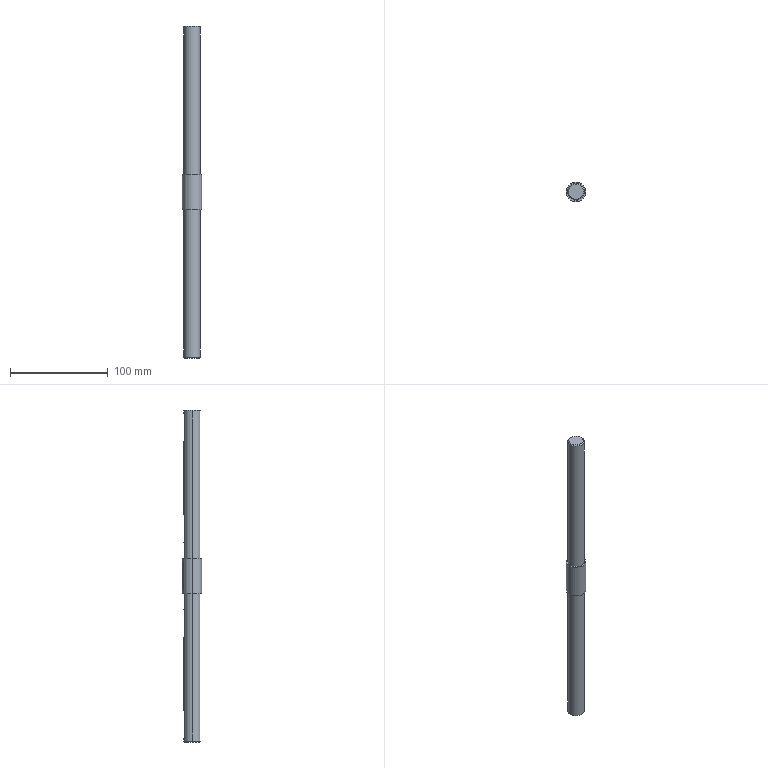Part | NX | features BREP 1, DATUM_CSYS 1, DATUM_PLANE 1, Delete Body 1, EXTRUDE 1, SKETCH 1 | 1 solid | 44 faces | box 20 x 20 x 340 mm | volume 77391 mm3 | cylinder 21 | plane 19 | cone 4 | commonest cylinder face diameters 6 x15 17 x4 20 x2
STEP:
#1=CARTESIAN_POINT('',(0.,8.5,-137.));
#2=VERTEX_POINT('',#1);
#3=CARTESIAN_POINT('',(0.,5.,-137.));
#4=VERTEX_POINT('',#3);
#5=CARTESIAN_POINT('',(0.,8.5,-137.));
#6=DIRECTION('',(0.,-1.,0.));
#7=VECTOR('',#6,1000.);
#8=LINE('',#5,#7);
#9=EDGE_CURVE('',#2,#4,#8,.T.);
#10=ORIENTED_EDGE('',*,*,#9,.F.);
#11=CARTESIAN_POINT('',(3.,7.953,-140.));
#12=VERTEX_POINT('',#11);
#13=CARTESIAN_POINT('',(0.,8.5,-137.));
#14=CARTESIAN_POINT('',(0.7993,8.5,-137.));
#15=CARTESIAN_POINT('',(2.343,8.236,-137.657));
#16=CARTESIAN_POINT('',(3.,7.953,-139.201));
#17=CARTESIAN_POINT('',(3.,7.953,-140.));
#18=B_SPLINE_CURVE_WITH_KNOTS('',3,(#13,#14,#15,#16,#17),.UNSPECIFIED.,.F.,.F.,(4,1,4),(0.,0.002363,0.004725),.UNSPECIFIED.);
#19=EDGE_CURVE('',#2,#12,#18,.T.);
#20=ORIENTED_EDGE('',*,*,#19,.T.);
#21=CARTESIAN_POINT('',(3.,5.,-140.));
#22=VERTEX_POINT('',#21);
#23=CARTESIAN_POINT('',(3.,7.953,-140.));
#24=DIRECTION('',(0.,-1.,0.));
#25=VECTOR('',#24,1000.);
#26=LINE('',#23,#25);
#27=EDGE_CURVE('',#12,#22,#26,.T.);
#28=ORIENTED_EDGE('',*,*,#27,.T.);
#29=CARTESIAN_POINT('',(0.,5.,-140.));
#30=DIRECTION('',(0.,1.,0.));
#31=DIRECTION('',(0.,0.,1.));
#32=AXIS2_PLACEMENT_3D('',#29,#30,#31);
#33=CIRCLE('',#32,3.);
#34=EDGE_CURVE('',#4,#22,#33,.T.);
#35=ORIENTED_EDGE('',*,*,#34,.F.);
#36=EDGE_LOOP('',(#10,#20,#28,#35));
#37=FACE_BOUND('',#36,.T.);
#38=CARTESIAN_POINT('',(0.,5.,-140.));
#39=DIRECTION('',(0.,1.,0.));
#40=DIRECTION('',(0.,0.,-1.));
#41=AXIS2_PLACEMENT_3D('',#38,#39,#40);
#42=CYLINDRICAL_SURFACE('',#41,3.);
#43=ADVANCED_FACE('',(#37),#42,.F.);
#44=CARTESIAN_POINT('',(0.,5.,-167.));
#45=VERTEX_POINT('',#44);
#46=CARTESIAN_POINT('',(-3.,5.,-164.));
#47=VERTEX_POINT('',#46);
#48=CARTESIAN_POINT('',(0.,5.,-164.));
#49=DIRECTION('',(0.,1.,0.));
#50=DIRECTION('',(0.,0.,-1.));
#51=AXIS2_PLACEMENT_3D('',#48,#49,#50);
#52=CIRCLE('',#51,3.);
#53=EDGE_CURVE('',#45,#47,#52,.T.);
#54=ORIENTED_EDGE('',*,*,#53,.T.);
#55=CARTESIAN_POINT('',(-3.,5.,-140.));
#56=VERTEX_POINT('',#55);
#57=CARTESIAN_POINT('',(-3.,5.,-140.));
#58=DIRECTION('',(0.,0.,-1.));
#59=VECTOR('',#58,1000.);
#60=LINE('',#57,#59);
#61=EDGE_CURVE('',#56,#47,#60,.T.);
#62=ORIENTED_EDGE('',*,*,#61,.F.);
#63=CARTESIAN_POINT('',(0.,5.,-140.));
#64=DIRECTION('',(0.,1.,0.));
#65=DIRECTION('',(-1.,0.,0.));
#66=AXIS2_PLACEMENT_3D('',#63,#64,#65);
#67=CIRCLE('',#66,3.);
#68=EDGE_CURVE('',#56,#4,#67,.T.);
#69=ORIENTED_EDGE('',*,*,#68,.T.);
#70=ORIENTED_EDGE('',*,*,#34,.T.);
#71=CARTESIAN_POINT('',(3.,5.,-164.));
#72=VERTEX_POINT('',#71);
#73=CARTESIAN_POINT('',(3.,5.,-164.));
#74=DIRECTION('',(0.,0.,1.));
#75=VECTOR('',#74,1000.);
#76=LINE('',#73,#75);
#77=EDGE_CURVE('',#72,#22,#76,.T.);
#78=ORIENTED_EDGE('',*,*,#77,.F.);
#79=CARTESIAN_POINT('',(0.,5.,-164.));
#80=DIRECTION('',(0.,1.,0.));
#81=DIRECTION('',(1.,0.,0.));
#82=AXIS2_PLACEMENT_3D('',#79,#80,#81);
#83=CIRCLE('',#82,3.);
#84=EDGE_CURVE('',#72,#45,#83,.T.);
#85=ORIENTED_EDGE('',*,*,#84,.T.);
#86=EDGE_LOOP('',(#54,#62,#69,#70,#78,#85));
#87=FACE_BOUND('',#86,.T.);
#88=CARTESIAN_POINT('',(0.,5.,-164.));
#89=DIRECTION('',(0.,1.,0.));
#90=DIRECTION('',(0.,0.,-1.));
#91=AXIS2_PLACEMENT_3D('',#88,#89,#90);
#92=PLANE('',#91);
#93=ADVANCED_FACE('',(#87),#92,.T.);
#94=ORIENTED_EDGE('',*,*,#53,.F.);
#95=ORIENTED_EDGE('',*,*,#84,.F.);
#96=CARTESIAN_POINT('',(3.,7.953,-164.));
#97=VERTEX_POINT('',#96);
#98=CARTESIAN_POINT('',(3.,5.,-164.));
#99=DIRECTION('',(0.,1.,0.));
#100=VECTOR('',#99,1000.);
#101=LINE('',#98,#100);
#102=EDGE_CURVE('',#72,#97,#101,.T.);
#103=ORIENTED_EDGE('',*,*,#102,.T.);
#104=CARTESIAN_POINT('',(0.,8.5,-167.));
#105=VERTEX_POINT('',#104);
#106=CARTESIAN_POINT('',(3.,7.953,-164.));
#107=CARTESIAN_POINT('',(3.,7.953,-164.799));
#108=CARTESIAN_POINT('',(2.344,8.235,-166.341));
#109=CARTESIAN_POINT('',(0.7993,8.5,-167.));
#110=CARTESIAN_POINT('',(0.,8.5,-167.));
#111=B_SPLINE_CURVE_WITH_KNOTS('',3,(#106,#107,#108,#109,#110),.UNSPECIFIED.,.F.,.F.,(4,1,4),(0.,0.002362,0.004725),.UNSPECIFIED.);
#112=EDGE_CURVE('',#97,#105,#111,.T.);
#113=ORIENTED_EDGE('',*,*,#112,.T.);
#114=CARTESIAN_POINT('',(-3.,7.953,-164.));
#115=VERTEX_POINT('',#114);
#116=CARTESIAN_POINT('',(0.,8.5,-167.));
#117=CARTESIAN_POINT('',(-0.7993,8.5,-167.));
#118=CARTESIAN_POINT('',(-2.343,8.236,-166.343));
#119=CARTESIAN_POINT('',(-3.,7.953,-164.799));
#120=CARTESIAN_POINT('',(-3.,7.953,-164.));
#121=B_SPLINE_CURVE_WITH_KNOTS('',3,(#116,#117,#118,#119,#120),.UNSPECIFIED.,.F.,.F.,(4,1,4),(0.,0.002363,0.004725),.UNSPECIFIED.);
#122=EDGE_CURVE('',#105,#115,#121,.T.);
#123=ORIENTED_EDGE('',*,*,#122,.T.);
#124=CARTESIAN_POINT('',(-3.,7.953,-164.));
#125=DIRECTION('',(0.,-1.,0.));
#126=VECTOR('',#125,1000.);
#127=LINE('',#124,#126);
#128=EDGE_CURVE('',#115,#47,#127,.T.);
#129=ORIENTED_EDGE('',*,*,#128,.T.);
#130=EDGE_LOOP('',(#94,#95,#103,#113,#123,#129));
#131=FACE_BOUND('',#130,.T.);
#132=CARTESIAN_POINT('',(0.,5.,-164.));
#133=DIRECTION('',(0.,1.,0.));
#134=DIRECTION('',(0.,0.,-1.));
#135=AXIS2_PLACEMENT_3D('',#132,#133,#134);
#136=CYLINDRICAL_SURFACE('',#135,3.);
#137=ADVANCED_FACE('',(#131),#136,.F.);
#138=ORIENTED_EDGE('',*,*,#61,.T.);
#139=ORIENTED_EDGE('',*,*,#128,.F.);
#140=CARTESIAN_POINT('',(-3.,7.953,-140.));
#141=VERTEX_POINT('',#140);
#142=CARTESIAN_POINT('',(-3.,7.953,-140.));
#143=DIRECTION('',(0.,0.,-1.));
#144=VECTOR('',#143,1000.);
#145=LINE('',#142,#144);
#146=EDGE_CURVE('',#141,#115,#145,.T.);
#147=ORIENTED_EDGE('',*,*,#146,.F.);
#148=CARTESIAN_POINT('',(-3.,5.,-140.));
#149=DIRECTION('',(0.,1.,0.));
#150=VECTOR('',#149,1000.);
#151=LINE('',#148,#150);
#152=EDGE_CURVE('',#56,#141,#151,.T.);
#153=ORIENTED_EDGE('',*,*,#152,.F.);
#154=EDGE_LOOP('',(#138,#139,#147,#153));
#155=FACE_BOUND('',#154,.T.);
#156=CARTESIAN_POINT('',(-3.,5.,-164.));
#157=DIRECTION('',(-1.,0.,0.));
#158=DIRECTION('',(0.,0.,-1.));
#159=AXIS2_PLACEMENT_3D('',#156,#157,#158);
#160=PLANE('',#159);
#161=ADVANCED_FACE('',(#155),#160,.F.);
#162=ORIENTED_EDGE('',*,*,#68,.F.);
#163=ORIENTED_EDGE('',*,*,#152,.T.);
#164=CARTESIAN_POINT('',(-3.,7.953,-140.));
#165=CARTESIAN_POINT('',(-3.,7.953,-139.201));
#166=CARTESIAN_POINT('',(-2.344,8.235,-137.659));
#167=CARTESIAN_POINT('',(-0.7993,8.5,-137.));
#168=CARTESIAN_POINT('',(0.,8.5,-137.));
#169=B_SPLINE_CURVE_WITH_KNOTS('',3,(#164,#165,#166,#167,#168),.UNSPECIFIED.,.F.,.F.,(4,1,4),(0.,0.002362,0.004725),.UNSPECIFIED.);
#170=EDGE_CURVE('',#141,#2,#169,.T.);
#171=ORIENTED_EDGE('',*,*,#170,.T.);
#172=ORIENTED_EDGE('',*,*,#9,.T.);
#173=EDGE_LOOP('',(#162,#163,#171,#172));
#174=FACE_BOUND('',#173,.T.);
#175=CARTESIAN_POINT('',(0.,5.,-140.));
#176=DIRECTION('',(0.,1.,0.));
#177=DIRECTION('',(0.,0.,-1.));
#178=AXIS2_PLACEMENT_3D('',#175,#176,#177);
#179=CYLINDRICAL_SURFACE('',#178,3.);
#180=ADVANCED_FACE('',(#174),#179,.F.);
#181=CARTESIAN_POINT('',(8.5,0.,-169.));
#182=VERTEX_POINT('',#181);
#183=CARTESIAN_POINT('',(8.5,0.,-18.));
#184=VERTEX_POINT('',#183);
#185=CARTESIAN_POINT('',(8.5,0.,-169.));
#186=DIRECTION('',(0.,0.,1.));
#187=VECTOR('',#186,1000.);
#188=LINE('',#185,#187);
#189=EDGE_CURVE('',#182,#184,#188,.T.);
#190=ORIENTED_EDGE('',*,*,#189,.F.);
#191=CARTESIAN_POINT('',(-8.5,0.,-169.));
#192=VERTEX_POINT('',#191);
#193=CARTESIAN_POINT('',(0.,0.,-169.));
#194=DIRECTION('',(0.,0.,-1.));
#195=DIRECTION('',(-1.,0.,0.));
#196=AXIS2_PLACEMENT_3D('',#193,#194,#195);
#197=CIRCLE('',#196,8.5);
#198=EDGE_CURVE('',#192,#182,#197,.T.);
#199=ORIENTED_EDGE('',*,*,#198,.F.);
#200=CARTESIAN_POINT('',(-8.5,0.,-18.));
#201=VERTEX_POINT('',#200);
#202=CARTESIAN_POINT('',(-8.5,0.,-169.));
#203=DIRECTION('',(0.,0.,1.));
#204=VECTOR('',#203,1000.);
#205=LINE('',#202,#204);
#206=EDGE_CURVE('',#192,#201,#205,.T.);
#207=ORIENTED_EDGE('',*,*,#206,.T.);
#208=CARTESIAN_POINT('',(0.,0.,-18.));
#209=DIRECTION('',(0.,0.,1.));
#210=DIRECTION('',(1.,0.,0.));
#211=AXIS2_PLACEMENT_3D('',#208,#209,#210);
#212=CIRCLE('',#211,8.5);
#213=EDGE_CURVE('',#184,#201,#212,.T.);
#214=ORIENTED_EDGE('',*,*,#213,.F.);
#215=EDGE_LOOP('',(#190,#199,#207,#214));
#216=FACE_BOUND('',#215,.T.);
#217=CARTESIAN_POINT('',(-3.,7.953,-37.));
#218=VERTEX_POINT('',#217);
#219=CARTESIAN_POINT('',(0.,8.5,-34.));
#220=VERTEX_POINT('',#219);
#221=CARTESIAN_POINT('',(-3.,7.953,-37.));
#222=CARTESIAN_POINT('',(-3.,7.953,-36.201));
#223=CARTESIAN_POINT('',(-2.344,8.235,-34.659));
#224=CARTESIAN_POINT('',(-0.7993,8.5,-34.));
#225=CARTESIAN_POINT('',(0.,8.5,-34.));
#226=B_SPLINE_CURVE_WITH_KNOTS('',3,(#221,#222,#223,#224,#225),.UNSPECIFIED.,.F.,.F.,(4,1,4),(0.,0.002362,0.004725),.UNSPECIFIED.);
#227=EDGE_CURVE('',#218,#220,#226,.T.);
#228=ORIENTED_EDGE('',*,*,#227,.F.);
#229=CARTESIAN_POINT('',(-3.,7.953,-61.));
#230=VERTEX_POINT('',#229);
#231=CARTESIAN_POINT('',(-3.,7.953,-37.));
#232=DIRECTION('',(0.,0.,-1.));
#233=VECTOR('',#232,1000.);
#234=LINE('',#231,#233);
#235=EDGE_CURVE('',#218,#230,#234,.T.);
#236=ORIENTED_EDGE('',*,*,#235,.T.);
#237=CARTESIAN_POINT('',(0.,8.5,-64.));
#238=VERTEX_POINT('',#237);
#239=CARTESIAN_POINT('',(0.,8.5,-64.));
#240=CARTESIAN_POINT('',(-0.7993,8.5,-64.));
#241=CARTESIAN_POINT('',(-2.343,8.236,-63.343));
#242=CARTESIAN_POINT('',(-3.,7.953,-61.799));
#243=CARTESIAN_POINT('',(-3.,7.953,-61.));
#244=B_SPLINE_CURVE_WITH_KNOTS('',3,(#239,#240,#241,#242,#243),.UNSPECIFIED.,.F.,.F.,(4,1,4),(0.,0.002363,0.004725),.UNSPECIFIED.);
#245=EDGE_CURVE('',#238,#230,#244,.T.);
#246=ORIENTED_EDGE('',*,*,#245,.F.);
#247=CARTESIAN_POINT('',(3.,7.953,-61.));
#248=VERTEX_POINT('',#247);
#249=CARTESIAN_POINT('',(3.,7.953,-61.));
#250=CARTESIAN_POINT('',(3.,7.953,-61.799));
#251=CARTESIAN_POINT('',(2.344,8.235,-63.341));
#252=CARTESIAN_POINT('',(0.7993,8.5,-64.));
#253=CARTESIAN_POINT('',(0.,8.5,-64.));
#254=B_SPLINE_CURVE_WITH_KNOTS('',3,(#249,#250,#251,#252,#253),.UNSPECIFIED.,.F.,.F.,(4,1,4),(0.,0.002362,0.004725),.UNSPECIFIED.);
#255=EDGE_CURVE('',#248,#238,#254,.T.);
#256=ORIENTED_EDGE('',*,*,#255,.F.);
#257=CARTESIAN_POINT('',(3.,7.953,-37.));
#258=VERTEX_POINT('',#257);
#259=CARTESIAN_POINT('',(3.,7.953,-61.));
#260=DIRECTION('',(0.,0.,1.));
#261=VECTOR('',#260,1000.);
#262=LINE('',#259,#261);
#263=EDGE_CURVE('',#248,#258,#262,.T.);
#264=ORIENTED_EDGE('',*,*,#263,.T.);
#265=CARTESIAN_POINT('',(0.,8.5,-34.));
#266=CARTESIAN_POINT('',(0.7993,8.5,-34.));
#267=CARTESIAN_POINT('',(2.343,8.236,-34.657));
#268=CARTESIAN_POINT('',(3.,7.953,-36.201));
#269=CARTESIAN_POINT('',(3.,7.953,-37.));
#270=B_SPLINE_CURVE_WITH_KNOTS('',3,(#265,#266,#267,#268,#269),.UNSPECIFIED.,.F.,.F.,(4,1,4),(0.,0.002363,0.004725),.UNSPECIFIED.);
#271=EDGE_CURVE('',#220,#258,#270,.T.);
#272=ORIENTED_EDGE('',*,*,#271,.F.);
#273=EDGE_LOOP('',(#228,#236,#246,#256,#264,#272));
#274=FACE_BOUND('',#273,.T.);
#275=ORIENTED_EDGE('',*,*,#170,.F.);
#276=ORIENTED_EDGE('',*,*,#146,.T.);
#277=ORIENTED_EDGE('',*,*,#122,.F.);
#278=ORIENTED_EDGE('',*,*,#112,.F.);
#279=CARTESIAN_POINT('',(3.,7.953,-164.));
#280=DIRECTION('',(0.,0.,1.));
#281=VECTOR('',#280,1000.);
#282=LINE('',#279,#281);
#283=EDGE_CURVE('',#97,#12,#282,.T.);
#284=ORIENTED_EDGE('',*,*,#283,.T.);
#285=ORIENTED_EDGE('',*,*,#19,.F.);
#286=EDGE_LOOP('',(#275,#276,#277,#278,#284,#285));
#287=FACE_BOUND('',#286,.T.);
#288=CARTESIAN_POINT('',(0.,0.,170.));
#289=DIRECTION('',(0.,0.,-1.));
#290=DIRECTION('',(1.,0.,0.));
#291=AXIS2_PLACEMENT_3D('',#288,#289,#290);
#292=CYLINDRICAL_SURFACE('',#291,8.5);
#293=ADVANCED_FACE('',(#216,#274,#287),#292,.T.);
#294=CARTESIAN_POINT('',(-10.,0.,-18.));
#295=VERTEX_POINT('',#294);
#296=CARTESIAN_POINT('',(10.,0.,-18.));
#297=VERTEX_POINT('',#296);
#298=CARTESIAN_POINT('',(0.,0.,-18.));
#299=DIRECTION('',(0.,0.,-1.));
#300=DIRECTION('',(-1.,0.,0.));
#301=AXIS2_PLACEMENT_3D('',#298,#299,#300);
#302=CIRCLE('',#301,10.);
#303=EDGE_CURVE('',#295,#297,#302,.T.);
#304=ORIENTED_EDGE('',*,*,#303,.T.);
#305=CARTESIAN_POINT('',(0.,0.,-18.));
#306=DIRECTION('',(0.,0.,-1.));
#307=DIRECTION('',(1.,0.,0.));
#308=AXIS2_PLACEMENT_3D('',#305,#306,#307);
#309=CIRCLE('',#308,10.);
#310=EDGE_CURVE('',#297,#295,#309,.T.);
#311=ORIENTED_EDGE('',*,*,#310,.T.);
#312=EDGE_LOOP('',(#304,#311));
#313=FACE_BOUND('',#312,.T.);
#314=ORIENTED_EDGE('',*,*,#213,.T.);
#315=CARTESIAN_POINT('',(0.,0.,-18.));
#316=DIRECTION('',(0.,0.,1.));
#317=DIRECTION('',(-1.,0.,0.));
#318=AXIS2_PLACEMENT_3D('',#315,#316,#317);
#319=CIRCLE('',#318,8.5);
#320=EDGE_CURVE('',#201,#184,#319,.T.);
#321=ORIENTED_EDGE('',*,*,#320,.T.);
#322=EDGE_LOOP('',(#314,#321));
#323=FACE_BOUND('',#322,.T.);
#324=CARTESIAN_POINT('',(0.,0.,-18.));
#325=DIRECTION('',(0.,0.,1.));
#326=DIRECTION('',(-1.,0.,0.));
#327=AXIS2_PLACEMENT_3D('',#324,#325,#326);
#328=PLANE('',#327);
#329=ADVANCED_FACE('',(#313,#323),#328,.F.);
#330=CARTESIAN_POINT('',(-10.,0.,18.));
#331=VERTEX_POINT('',#330);
#332=CARTESIAN_POINT('',(10.,0.,18.));
#333=VERTEX_POINT('',#332);
#334=CARTESIAN_POINT('',(0.,0.,18.));
#335=DIRECTION('',(0.,0.,1.));
#336=DIRECTION('',(-1.,0.,0.));
#337=AXIS2_PLACEMENT_3D('',#334,#335,#336);
#338=CIRCLE('',#337,10.);
#339=EDGE_CURVE('',#331,#333,#338,.T.);
#340=ORIENTED_EDGE('',*,*,#339,.F.);
#341=CARTESIAN_POINT('',(-10.,0.,-18.));
#342=DIRECTION('',(0.,0.,1.));
#343=VECTOR('',#342,1000.);
#344=LINE('',#341,#343);
#345=EDGE_CURVE('',#331,#295,#344,.F.);
#346=ORIENTED_EDGE('',*,*,#345,.T.);
#347=ORIENTED_EDGE('',*,*,#310,.F.);
#348=CARTESIAN_POINT('',(10.,0.,-18.));
#349=DIRECTION('',(0.,0.,1.));
#350=VECTOR('',#349,1000.);
#351=LINE('',#348,#350);
#352=EDGE_CURVE('',#333,#297,#351,.F.);
#353=ORIENTED_EDGE('',*,*,#352,.F.);
#354=EDGE_LOOP('',(#340,#346,#347,#353));
#355=FACE_BOUND('',#354,.T.);
#356=CARTESIAN_POINT('',(0.,0.,18.));
#357=DIRECTION('',(0.,0.,-1.));
#358=DIRECTION('',(1.,0.,0.));
#359=AXIS2_PLACEMENT_3D('',#356,#357,#358);
#360=CYLINDRICAL_SURFACE('',#359,10.);
#361=ADVANCED_FACE('',(#355),#360,.T.);
#362=ORIENTED_EDGE('',*,*,#352,.T.);
#363=ORIENTED_EDGE('',*,*,#303,.F.);
#364=ORIENTED_EDGE('',*,*,#345,.F.);
#365=CARTESIAN_POINT('',(0.,0.,18.));
#366=DIRECTION('',(0.,0.,1.));
#367=DIRECTION('',(1.,0.,0.));
#368=AXIS2_PLACEMENT_3D('',#365,#366,#367);
#369=CIRCLE('',#368,10.);
#370=EDGE_CURVE('',#333,#331,#369,.T.);
#371=ORIENTED_EDGE('',*,*,#370,.F.);
#372=EDGE_LOOP('',(#362,#363,#364,#371));
#373=FACE_BOUND('',#372,.T.);
#374=CARTESIAN_POINT('',(0.,10.,15.));
#375=VERTEX_POINT('',#374);
#376=CARTESIAN_POINT('',(3.,9.539,12.));
#377=VERTEX_POINT('',#376);
#378=CARTESIAN_POINT('',(0.,10.,15.));
#379=CARTESIAN_POINT('',(0.7973,10.,15.));
#380=CARTESIAN_POINT('',(2.343,9.775,14.345));
#381=CARTESIAN_POINT('',(3.,9.539,12.797));
#382=CARTESIAN_POINT('',(3.,9.539,12.));
#383=B_SPLINE_CURVE_WITH_KNOTS('',3,(#378,#379,#380,#381,#382),.UNSPECIFIED.,.F.,.F.,(4,1,4),(0.,0.002357,0.004714),.UNSPECIFIED.);
#384=EDGE_CURVE('',#375,#377,#383,.T.);
#385=ORIENTED_EDGE('',*,*,#384,.F.);
#386=CARTESIAN_POINT('',(-3.,9.539,12.));
#387=VERTEX_POINT('',#386);
#388=CARTESIAN_POINT('',(-3.,9.539,12.));
#389=CARTESIAN_POINT('',(-3.,9.539,12.797));
#390=CARTESIAN_POINT('',(-2.345,9.775,14.343));
#391=CARTESIAN_POINT('',(-0.7973,10.,15.));
#392=CARTESIAN_POINT('',(0.,10.,15.));
#393=B_SPLINE_CURVE_WITH_KNOTS('',3,(#388,#389,#390,#391,#392),.UNSPECIFIED.,.F.,.F.,(4,1,4),(0.,0.002357,0.004714),.UNSPECIFIED.);
#394=EDGE_CURVE('',#387,#375,#393,.T.);
#395=ORIENTED_EDGE('',*,*,#394,.F.);
#396=CARTESIAN_POINT('',(-3.,9.539,-12.));
#397=VERTEX_POINT('',#396);
#398=CARTESIAN_POINT('',(-3.,9.539,12.));
#399=DIRECTION('',(0.,0.,-1.));
#400=VECTOR('',#399,1000.);
#401=LINE('',#398,#400);
#402=EDGE_CURVE('',#387,#397,#401,.T.);
#403=ORIENTED_EDGE('',*,*,#402,.T.);
#404=CARTESIAN_POINT('',(0.,10.,-15.));
#405=VERTEX_POINT('',#404);
#406=CARTESIAN_POINT('',(0.,10.,-15.));
#407=CARTESIAN_POINT('',(-0.7973,10.,-15.));
#408=CARTESIAN_POINT('',(-2.343,9.775,-14.345));
#409=CARTESIAN_POINT('',(-3.,9.539,-12.797));
#410=CARTESIAN_POINT('',(-3.,9.539,-12.));
#411=B_SPLINE_CURVE_WITH_KNOTS('',3,(#406,#407,#408,#409,#410),.UNSPECIFIED.,.F.,.F.,(4,1,4),(0.,0.002357,0.004714),.UNSPECIFIED.);
#412=EDGE_CURVE('',#405,#397,#411,.T.);
#413=ORIENTED_EDGE('',*,*,#412,.F.);
#414=CARTESIAN_POINT('',(3.,9.539,-12.));
#415=VERTEX_POINT('',#414);
#416=CARTESIAN_POINT('',(3.,9.539,-12.));
#417=CARTESIAN_POINT('',(3.,9.539,-12.797));
#418=CARTESIAN_POINT('',(2.345,9.775,-14.343));
#419=CARTESIAN_POINT('',(0.7973,10.,-15.));
#420=CARTESIAN_POINT('',(0.,10.,-15.));
#421=B_SPLINE_CURVE_WITH_KNOTS('',3,(#416,#417,#418,#419,#420),.UNSPECIFIED.,.F.,.F.,(4,1,4),(0.,0.002357,0.004714),.UNSPECIFIED.);
#422=EDGE_CURVE('',#415,#405,#421,.T.);
#423=ORIENTED_EDGE('',*,*,#422,.F.);
#424=CARTESIAN_POINT('',(3.,9.539,-12.));
#425=DIRECTION('',(0.,0.,1.));
#426=VECTOR('',#425,1000.);
#427=LINE('',#424,#426);
#428=EDGE_CURVE('',#415,#377,#427,.T.);
#429=ORIENTED_EDGE('',*,*,#428,.T.);
#430=EDGE_LOOP('',(#385,#395,#403,#413,#423,#429));
#431=FACE_BOUND('',#430,.T.);
#432=CARTESIAN_POINT('',(0.,0.,18.));
#433=DIRECTION('',(0.,0.,-1.));
#434=DIRECTION('',(1.,0.,0.));
#435=AXIS2_PLACEMENT_3D('',#432,#433,#434);
#436=CYLINDRICAL_SURFACE('',#435,10.);
#437=ADVANCED_FACE('',(#373,#431),#436,.T.);
#438=ORIENTED_EDGE('',*,*,#370,.T.);
#439=ORIENTED_EDGE('',*,*,#339,.T.);
#440=EDGE_LOOP('',(#438,#439));
#441=FACE_BOUND('',#440,.T.);
#442=CARTESIAN_POINT('',(-8.5,0.,18.));
#443=VERTEX_POINT('',#442);
#444=CARTESIAN_POINT('',(8.5,0.,18.));
#445=VERTEX_POINT('',#444);
#446=CARTESIAN_POINT('',(0.,0.,18.));
#447=DIRECTION('',(0.,0.,-1.));
#448=DIRECTION('',(-1.,0.,0.));
#449=AXIS2_PLACEMENT_3D('',#446,#447,#448);
#450=CIRCLE('',#449,8.5);
#451=EDGE_CURVE('',#443,#445,#450,.T.);
#452=ORIENTED_EDGE('',*,*,#451,.T.);
#453=CARTESIAN_POINT('',(0.,0.,18.));
#454=DIRECTION('',(0.,0.,-1.));
#455=DIRECTION('',(1.,0.,0.));
#456=AXIS2_PLACEMENT_3D('',#453,#454,#455);
#457=CIRCLE('',#456,8.5);
#458=EDGE_CURVE('',#445,#443,#457,.T.);
#459=ORIENTED_EDGE('',*,*,#458,.T.);
#460=EDGE_LOOP('',(#452,#459));
#461=FACE_BOUND('',#460,.T.);
#462=CARTESIAN_POINT('',(0.,0.,18.));
#463=DIRECTION('',(0.,0.,1.));
#464=DIRECTION('',(-1.,0.,0.));
#465=AXIS2_PLACEMENT_3D('',#462,#463,#464);
#466=PLANE('',#465);
#467=ADVANCED_FACE('',(#441,#461),#466,.T.);
#468=CARTESIAN_POINT('',(-8.5,0.,169.));
#469=VERTEX_POINT('',#468);
#470=CARTESIAN_POINT('',(8.5,0.,169.));
#471=VERTEX_POINT('',#470);
#472=CARTESIAN_POINT('',(0.,0.,169.));
#473=DIRECTION('',(0.,0.,1.));
#474=DIRECTION('',(-1.,0.,0.));
#475=AXIS2_PLACEMENT_3D('',#472,#473,#474);
#476=CIRCLE('',#475,8.5);
#477=EDGE_CURVE('',#469,#471,#476,.T.);
#478=ORIENTED_EDGE('',*,*,#477,.F.);
#479=CARTESIAN_POINT('',(-8.5,0.,18.));
#480=DIRECTION('',(0.,0.,1.));
#481=VECTOR('',#480,1000.);
#482=LINE('',#479,#481);
#483=EDGE_CURVE('',#469,#443,#482,.F.);
#484=ORIENTED_EDGE('',*,*,#483,.T.);
#485=ORIENTED_EDGE('',*,*,#458,.F.);
#486=CARTESIAN_POINT('',(8.5,0.,18.));
#487=DIRECTION('',(0.,0.,1.));
#488=VECTOR('',#487,1000.);
#489=LINE('',#486,#488);
#490=EDGE_CURVE('',#471,#445,#489,.F.);
#491=ORIENTED_EDGE('',*,*,#490,.F.);
#492=EDGE_LOOP('',(#478,#484,#485,#491));
#493=FACE_BOUND('',#492,.T.);
#494=CARTESIAN_POINT('',(0.,0.,170.));
#495=DIRECTION('',(0.,0.,-1.));
#496=DIRECTION('',(1.,0.,0.));
#497=AXIS2_PLACEMENT_3D('',#494,#495,#496);
#498=CYLINDRICAL_SURFACE('',#497,8.5);
#499=ADVANCED_FACE('',(#493),#498,.T.);
#500=ORIENTED_EDGE('',*,*,#490,.T.);
#501=ORIENTED_EDGE('',*,*,#451,.F.);
#502=ORIENTED_EDGE('',*,*,#483,.F.);
#503=CARTESIAN_POINT('',(0.,0.,169.));
#504=DIRECTION('',(0.,0.,1.));
#505=DIRECTION('',(1.,0.,0.));
#506=AXIS2_PLACEMENT_3D('',#503,#504,#505);
#507=CIRCLE('',#506,8.5);
#508=EDGE_CURVE('',#471,#469,#507,.T.);
#509=ORIENTED_EDGE('',*,*,#508,.F.);
#510=EDGE_LOOP('',(#500,#501,#502,#509));
#511=FACE_BOUND('',#510,.T.);
#512=CARTESIAN_POINT('',(-3.,7.953,164.));
#513=VERTEX_POINT('',#512);
#514=CARTESIAN_POINT('',(0.,8.5,167.));
#515=VERTEX_POINT('',#514);
#516=CARTESIAN_POINT('',(-3.,7.953,164.));
#517=CARTESIAN_POINT('',(-3.,7.953,164.799));
#518=CARTESIAN_POINT('',(-2.344,8.235,166.341));
#519=CARTESIAN_POINT('',(-0.7993,8.5,167.));
#520=CARTESIAN_POINT('',(0.,8.5,167.));
#521=B_SPLINE_CURVE_WITH_KNOTS('',3,(#516,#517,#518,#519,#520),.UNSPECIFIED.,.F.,.F.,(4,1,4),(0.,0.002362,0.004725),.UNSPECIFIED.);
#522=EDGE_CURVE('',#513,#515,#521,.T.);
#523=ORIENTED_EDGE('',*,*,#522,.F.);
#524=CARTESIAN_POINT('',(-3.,7.953,140.));
#525=VERTEX_POINT('',#524);
#526=CARTESIAN_POINT('',(-3.,7.953,164.));
#527=DIRECTION('',(0.,0.,-1.));
#528=VECTOR('',#527,1000.);
#529=LINE('',#526,#528);
#530=EDGE_CURVE('',#513,#525,#529,.T.);
#531=ORIENTED_EDGE('',*,*,#530,.T.);
#532=CARTESIAN_POINT('',(0.,8.5,137.));
#533=VERTEX_POINT('',#532);
#534=CARTESIAN_POINT('',(0.,8.5,137.));
#535=CARTESIAN_POINT('',(-0.7993,8.5,137.));
#536=CARTESIAN_POINT('',(-2.343,8.236,137.657));
#537=CARTESIAN_POINT('',(-3.,7.953,139.201));
#538=CARTESIAN_POINT('',(-3.,7.953,140.));
#539=B_SPLINE_CURVE_WITH_KNOTS('',3,(#534,#535,#536,#537,#538),.UNSPECIFIED.,.F.,.F.,(4,1,4),(0.,0.002363,0.004725),.UNSPECIFIED.);
#540=EDGE_CURVE('',#533,#525,#539,.T.);
#541=ORIENTED_EDGE('',*,*,#540,.F.);
#542=CARTESIAN_POINT('',(3.,7.953,140.));
#543=VERTEX_POINT('',#542);
#544=CARTESIAN_POINT('',(3.,7.953,140.));
#545=CARTESIAN_POINT('',(3.,7.953,139.201));
#546=CARTESIAN_POINT('',(2.344,8.235,137.659));
#547=CARTESIAN_POINT('',(0.7993,8.5,137.));
#548=CARTESIAN_POINT('',(0.,8.5,137.));
#549=B_SPLINE_CURVE_WITH_KNOTS('',3,(#544,#545,#546,#547,#548),.UNSPECIFIED.,.F.,.F.,(4,1,4),(0.,0.002362,0.004725),.UNSPECIFIED.);
#550=EDGE_CURVE('',#543,#533,#549,.T.);
#551=ORIENTED_EDGE('',*,*,#550,.F.);
#552=CARTESIAN_POINT('',(3.,7.953,164.));
#553=VERTEX_POINT('',#552);
#554=CARTESIAN_POINT('',(3.,7.953,140.));
#555=DIRECTION('',(0.,0.,1.));
#556=VECTOR('',#555,1000.);
#557=LINE('',#554,#556);
#558=EDGE_CURVE('',#543,#553,#557,.T.);
#559=ORIENTED_EDGE('',*,*,#558,.T.);
#560=CARTESIAN_POINT('',(0.,8.5,167.));
#561=CARTESIAN_POINT('',(0.7993,8.5,167.));
#562=CARTESIAN_POINT('',(2.343,8.236,166.343));
#563=CARTESIAN_POINT('',(3.,7.953,164.799));
#564=CARTESIAN_POINT('',(3.,7.953,164.));
#565=B_SPLINE_CURVE_WITH_KNOTS('',3,(#560,#561,#562,#563,#564),.UNSPECIFIED.,.F.,.F.,(4,1,4),(0.,0.002363,0.004725),.UNSPECIFIED.);
#566=EDGE_CURVE('',#515,#553,#565,.T.);
#567=ORIENTED_EDGE('',*,*,#566,.F.);
#568=EDGE_LOOP('',(#523,#531,#541,#551,#559,#567));
#569=FACE_BOUND('',#568,.T.);
#570=CARTESIAN_POINT('',(-3.,7.953,61.));
#571=VERTEX_POINT('',#570);
#572=CARTESIAN_POINT('',(0.,8.5,64.));
#573=VERTEX_POINT('',#572);
#574=CARTESIAN_POINT('',(-3.,7.953,61.));
#575=CARTESIAN_POINT('',(-3.,7.953,61.799));
#576=CARTESIAN_POINT('',(-2.344,8.235,63.341));
#577=CARTESIAN_POINT('',(-0.7993,8.5,64.));
#578=CARTESIAN_POINT('',(0.,8.5,64.));
#579=B_SPLINE_CURVE_WITH_KNOTS('',3,(#574,#575,#576,#577,#578),.UNSPECIFIED.,.F.,.F.,(4,1,4),(0.,0.002362,0.004725),.UNSPECIFIED.);
#580=EDGE_CURVE('',#571,#573,#579,.T.);
#581=ORIENTED_EDGE('',*,*,#580,.F.);
#582=CARTESIAN_POINT('',(-3.,7.953,37.));
#583=VERTEX_POINT('',#582);
#584=CARTESIAN_POINT('',(-3.,7.953,61.));
#585=DIRECTION('',(0.,0.,-1.));
#586=VECTOR('',#585,1000.);
#587=LINE('',#584,#586);
#588=EDGE_CURVE('',#571,#583,#587,.T.);
#589=ORIENTED_EDGE('',*,*,#588,.T.);
#590=CARTESIAN_POINT('',(3.,7.953,37.));
#591=VERTEX_POINT('',#590);
#592=CARTESIAN_POINT('',(3.,7.953,37.));
#593=CARTESIAN_POINT('',(3.,7.953,36.2));
#594=CARTESIAN_POINT('',(2.35,8.235,34.658));
#595=CARTESIAN_POINT('',(0.005449,8.632,33.671));
#596=CARTESIAN_POINT('',(-2.352,8.236,34.656));
#597=CARTESIAN_POINT('',(-3.,7.953,36.2));
#598=CARTESIAN_POINT('',(-3.,7.953,37.));
#599=B_SPLINE_CURVE_WITH_KNOTS('',3,(#592,#593,#594,#595,#596,#597,#598),.UNSPECIFIED.,.F.,.F.,(4,1,1,1,4),(0.,0.002363,0.004726,0.007089,0.009452),.UNSPECIFIED.);
#600=EDGE_CURVE('',#591,#583,#599,.T.);
#601=ORIENTED_EDGE('',*,*,#600,.F.);
#602=CARTESIAN_POINT('',(3.,7.953,61.));
#603=VERTEX_POINT('',#602);
#604=CARTESIAN_POINT('',(3.,7.953,37.));
#605=DIRECTION('',(0.,0.,1.));
#606=VECTOR('',#605,1000.);
#607=LINE('',#604,#606);
#608=EDGE_CURVE('',#591,#603,#607,.T.);
#609=ORIENTED_EDGE('',*,*,#608,.T.);
#610=CARTESIAN_POINT('',(0.,8.5,64.));
#611=CARTESIAN_POINT('',(0.7993,8.5,64.));
#612=CARTESIAN_POINT('',(2.343,8.236,63.343));
#613=CARTESIAN_POINT('',(3.,7.953,61.799));
#614=CARTESIAN_POINT('',(3.,7.953,61.));
#615=B_SPLINE_CURVE_WITH_KNOTS('',3,(#610,#611,#612,#613,#614),.UNSPECIFIED.,.F.,.F.,(4,1,4),(0.,0.002363,0.004725),.UNSPECIFIED.);
#616=EDGE_CURVE('',#573,#603,#615,.T.);
#617=ORIENTED_EDGE('',*,*,#616,.F.);
#618=EDGE_LOOP('',(#581,#589,#601,#609,#617));
#619=FACE_BOUND('',#618,.T.);
#620=CARTESIAN_POINT('',(0.,0.,170.));
#621=DIRECTION('',(0.,0.,-1.));
#622=DIRECTION('',(1.,0.,0.));
#623=AXIS2_PLACEMENT_3D('',#620,#621,#622);
#624=CYLINDRICAL_SURFACE('',#623,8.5);
#625=ADVANCED_FACE('',(#511,#569,#619),#624,.T.);
#626=CARTESIAN_POINT('',(7.5,0.,170.));
#627=VERTEX_POINT('',#626);
#628=CARTESIAN_POINT('',(8.5,0.,169.));
#629=DIRECTION('',(-0.7071,0.,0.7071));
#630=VECTOR('',#629,1000.);
#631=LINE('',#628,#630);
#632=EDGE_CURVE('',#471,#627,#631,.T.);
#633=ORIENTED_EDGE('',*,*,#632,.F.);
#634=ORIENTED_EDGE('',*,*,#508,.T.);
#635=CARTESIAN_POINT('',(-7.5,0.,170.));
#636=VERTEX_POINT('',#635);
#637=CARTESIAN_POINT('',(-8.5,0.,169.));
#638=DIRECTION('',(0.7071,0.,0.7071));
#639=VECTOR('',#638,1000.);
#640=LINE('',#637,#639);
#641=EDGE_CURVE('',#469,#636,#640,.T.);
#642=ORIENTED_EDGE('',*,*,#641,.T.);
#643=CARTESIAN_POINT('',(0.,0.,170.));
#644=DIRECTION('',(0.,0.,1.));
#645=DIRECTION('',(1.,0.,0.));
#646=AXIS2_PLACEMENT_3D('',#643,#644,#645);
#647=CIRCLE('',#646,7.5);
#648=EDGE_CURVE('',#627,#636,#647,.T.);
#649=ORIENTED_EDGE('',*,*,#648,.F.);
#650=EDGE_LOOP('',(#633,#634,#642,#649));
#651=FACE_BOUND('',#650,.T.);
#652=CARTESIAN_POINT('',(0.,0.,169.5));
#653=DIRECTION('',(0.,0.,-1.));
#654=DIRECTION('',(1.,0.,0.));
#655=AXIS2_PLACEMENT_3D('',#652,#653,#654);
#656=CONICAL_SURFACE('',#655,8.,0.7854);
#657=ADVANCED_FACE('',(#651),#656,.T.);
#658=ORIENTED_EDGE('',*,*,#648,.T.);
#659=CARTESIAN_POINT('',(0.,0.,170.));
#660=DIRECTION('',(0.,0.,1.));
#661=DIRECTION('',(-1.,0.,0.));
#662=AXIS2_PLACEMENT_3D('',#659,#660,#661);
#663=CIRCLE('',#662,7.5);
#664=EDGE_CURVE('',#636,#627,#663,.T.);
#665=ORIENTED_EDGE('',*,*,#664,.T.);
#666=EDGE_LOOP('',(#658,#665));
#667=FACE_BOUND('',#666,.T.);
#668=CARTESIAN_POINT('',(0.,0.,170.));
#669=DIRECTION('',(0.,0.,1.));
#670=DIRECTION('',(-1.,0.,0.));
#671=AXIS2_PLACEMENT_3D('',#668,#669,#670);
#672=PLANE('',#671);
#673=ADVANCED_FACE('',(#667),#672,.T.);
#674=ORIENTED_EDGE('',*,*,#664,.F.);
#675=ORIENTED_EDGE('',*,*,#641,.F.);
#676=ORIENTED_EDGE('',*,*,#477,.T.);
#677=ORIENTED_EDGE('',*,*,#632,.T.);
#678=EDGE_LOOP('',(#674,#675,#676,#677));
#679=FACE_BOUND('',#678,.T.);
#680=CARTESIAN_POINT('',(0.,0.,169.5));
#681=DIRECTION('',(0.,0.,-1.));
#682=DIRECTION('',(1.,0.,0.));
#683=AXIS2_PLACEMENT_3D('',#680,#681,#682);
#684=CONICAL_SURFACE('',#683,8.,0.7854);
#685=ADVANCED_FACE('',(#679),#684,.T.);
#686=CARTESIAN_POINT('',(0.,5.,167.));
#687=VERTEX_POINT('',#686);
#688=CARTESIAN_POINT('',(0.,8.5,167.));
#689=DIRECTION('',(0.,-1.,0.));
#690=VECTOR('',#689,1000.);
#691=LINE('',#688,#690);
#692=EDGE_CURVE('',#515,#687,#691,.T.);
#693=ORIENTED_EDGE('',*,*,#692,.F.);
#694=ORIENTED_EDGE('',*,*,#566,.T.);
#695=CARTESIAN_POINT('',(3.,5.,164.));
#696=VERTEX_POINT('',#695);
#697=CARTESIAN_POINT('',(3.,7.953,164.));
#698=DIRECTION('',(0.,-1.,0.));
#699=VECTOR('',#698,1000.);
#700=LINE('',#697,#699);
#701=EDGE_CURVE('',#553,#696,#700,.T.);
#702=ORIENTED_EDGE('',*,*,#701,.T.);
#703=CARTESIAN_POINT('',(0.,5.,164.));
#704=DIRECTION('',(0.,1.,0.));
#705=DIRECTION('',(0.,0.,1.));
#706=AXIS2_PLACEMENT_3D('',#703,#704,#705);
#707=CIRCLE('',#706,3.);
#708=EDGE_CURVE('',#687,#696,#707,.T.);
#709=ORIENTED_EDGE('',*,*,#708,.F.);
#710=EDGE_LOOP('',(#693,#694,#702,#709));
#711=FACE_BOUND('',#710,.T.);
#712=CARTESIAN_POINT('',(0.,5.,164.));
#713=DIRECTION('',(0.,1.,0.));
#714=DIRECTION('',(0.,0.,-1.));
#715=AXIS2_PLACEMENT_3D('',#712,#713,#714);
#716=CYLINDRICAL_SURFACE('',#715,3.);
#717=ADVANCED_FACE('',(#711),#716,.F.);
#718=ORIENTED_EDGE('',*,*,#708,.T.);
#719=CARTESIAN_POINT('',(3.,5.,140.));
#720=VERTEX_POINT('',#719);
#721=CARTESIAN_POINT('',(3.,5.,140.));
#722=DIRECTION('',(0.,0.,1.));
#723=VECTOR('',#722,1000.);
#724=LINE('',#721,#723);
#725=EDGE_CURVE('',#720,#696,#724,.T.);
#726=ORIENTED_EDGE('',*,*,#725,.F.);
#727=CARTESIAN_POINT('',(-3.,5.,140.));
#728=VERTEX_POINT('',#727);
#729=CARTESIAN_POINT('',(0.,5.,140.));
#730=DIRECTION('',(0.,1.,0.));
#731=DIRECTION('',(1.,0.,0.));
#732=AXIS2_PLACEMENT_3D('',#729,#730,#731);
#733=CIRCLE('',#732,3.);
#734=EDGE_CURVE('',#720,#728,#733,.T.);
#735=ORIENTED_EDGE('',*,*,#734,.T.);
#736=CARTESIAN_POINT('',(-3.,5.,164.));
#737=VERTEX_POINT('',#736);
#738=CARTESIAN_POINT('',(-3.,5.,164.));
#739=DIRECTION('',(0.,0.,-1.));
#740=VECTOR('',#739,1000.);
#741=LINE('',#738,#740);
#742=EDGE_CURVE('',#737,#728,#741,.T.);
#743=ORIENTED_EDGE('',*,*,#742,.F.);
#744=CARTESIAN_POINT('',(0.,5.,164.));
#745=DIRECTION('',(0.,1.,0.));
#746=DIRECTION('',(-1.,0.,0.));
#747=AXIS2_PLACEMENT_3D('',#744,#745,#746);
#748=CIRCLE('',#747,3.);
#749=EDGE_CURVE('',#737,#687,#748,.T.);
#750=ORIENTED_EDGE('',*,*,#749,.T.);
#751=EDGE_LOOP('',(#718,#726,#735,#743,#750));
#752=FACE_BOUND('',#751,.T.);
#753=CARTESIAN_POINT('',(0.,5.,164.));
#754=DIRECTION('',(0.,-1.,0.));
#755=DIRECTION('',(0.,0.,1.));
#756=AXIS2_PLACEMENT_3D('',#753,#754,#755);
#757=PLANE('',#756);
#758=ADVANCED_FACE('',(#752),#757,.F.);
#759=ORIENTED_EDGE('',*,*,#749,.F.);
#760=CARTESIAN_POINT('',(-3.,5.,164.));
#761=DIRECTION('',(0.,1.,0.));
#762=VECTOR('',#761,1000.);
#763=LINE('',#760,#762);
#764=EDGE_CURVE('',#737,#513,#763,.T.);
#765=ORIENTED_EDGE('',*,*,#764,.T.);
#766=ORIENTED_EDGE('',*,*,#522,.T.);
#767=ORIENTED_EDGE('',*,*,#692,.T.);
#768=EDGE_LOOP('',(#759,#765,#766,#767));
#769=FACE_BOUND('',#768,.T.);
#770=CARTESIAN_POINT('',(0.,5.,164.));
#771=DIRECTION('',(0.,1.,0.));
#772=DIRECTION('',(0.,0.,-1.));
#773=AXIS2_PLACEMENT_3D('',#770,#771,#772);
#774=CYLINDRICAL_SURFACE('',#773,3.);
#775=ADVANCED_FACE('',(#769),#774,.F.);
#776=ORIENTED_EDGE('',*,*,#742,.T.);
#777=CARTESIAN_POINT('',(-3.,7.953,140.));
#778=DIRECTION('',(0.,-1.,0.));
#779=VECTOR('',#778,1000.);
#780=LINE('',#777,#779);
#781=EDGE_CURVE('',#525,#728,#780,.T.);
#782=ORIENTED_EDGE('',*,*,#781,.F.);
#783=ORIENTED_EDGE('',*,*,#530,.F.);
#784=ORIENTED_EDGE('',*,*,#764,.F.);
#785=EDGE_LOOP('',(#776,#782,#783,#784));
#786=FACE_BOUND('',#785,.T.);
#787=CARTESIAN_POINT('',(-3.,5.,164.));
#788=DIRECTION('',(-1.,0.,0.));
#789=DIRECTION('',(0.,0.,-1.));
#790=AXIS2_PLACEMENT_3D('',#787,#788,#789);
#791=PLANE('',#790);
#792=ADVANCED_FACE('',(#786),#791,.F.);
#793=ORIENTED_EDGE('',*,*,#734,.F.);
#794=CARTESIAN_POINT('',(3.,5.,140.));
#795=DIRECTION('',(0.,1.,0.));
#796=VECTOR('',#795,1000.);
#797=LINE('',#794,#796);
#798=EDGE_CURVE('',#720,#543,#797,.T.);
#799=ORIENTED_EDGE('',*,*,#798,.T.);
#800=ORIENTED_EDGE('',*,*,#550,.T.);
#801=ORIENTED_EDGE('',*,*,#540,.T.);
#802=ORIENTED_EDGE('',*,*,#781,.T.);
#803=EDGE_LOOP('',(#793,#799,#800,#801,#802));
#804=FACE_BOUND('',#803,.T.);
#805=CARTESIAN_POINT('',(0.,5.,140.));
#806=DIRECTION('',(0.,1.,0.));
#807=DIRECTION('',(0.,0.,-1.));
#808=AXIS2_PLACEMENT_3D('',#805,#806,#807);
#809=CYLINDRICAL_SURFACE('',#808,3.);
#810=ADVANCED_FACE('',(#804),#809,.F.);
#811=ORIENTED_EDGE('',*,*,#725,.T.);
#812=ORIENTED_EDGE('',*,*,#701,.F.);
#813=ORIENTED_EDGE('',*,*,#558,.F.);
#814=ORIENTED_EDGE('',*,*,#798,.F.);
#815=EDGE_LOOP('',(#811,#812,#813,#814));
#816=FACE_BOUND('',#815,.T.);
#817=CARTESIAN_POINT('',(3.,5.,164.));
#818=DIRECTION('',(1.,0.,0.));
#819=DIRECTION('',(0.,0.,1.));
#820=AXIS2_PLACEMENT_3D('',#817,#818,#819);
#821=PLANE('',#820);
#822=ADVANCED_FACE('',(#816),#821,.F.);
#823=CARTESIAN_POINT('',(0.,5.,64.));
#824=VERTEX_POINT('',#823);
#825=CARTESIAN_POINT('',(0.,8.5,64.));
#826=DIRECTION('',(0.,-1.,0.));
#827=VECTOR('',#826,1000.);
#828=LINE('',#825,#827);
#829=EDGE_CURVE('',#573,#824,#828,.T.);
#830=ORIENTED_EDGE('',*,*,#829,.F.);
#831=ORIENTED_EDGE('',*,*,#616,.T.);
#832=CARTESIAN_POINT('',(3.,5.,61.));
#833=VERTEX_POINT('',#832);
#834=CARTESIAN_POINT('',(3.,7.953,61.));
#835=DIRECTION('',(0.,-1.,0.));
#836=VECTOR('',#835,1000.);
#837=LINE('',#834,#836);
#838=EDGE_CURVE('',#603,#833,#837,.T.);
#839=ORIENTED_EDGE('',*,*,#838,.T.);
#840=CARTESIAN_POINT('',(0.,5.,61.));
#841=DIRECTION('',(0.,1.,0.));
#842=DIRECTION('',(0.,0.,1.));
#843=AXIS2_PLACEMENT_3D('',#840,#841,#842);
#844=CIRCLE('',#843,3.);
#845=EDGE_CURVE('',#824,#833,#844,.T.);
#846=ORIENTED_EDGE('',*,*,#845,.F.);
#847=EDGE_LOOP('',(#830,#831,#839,#846));
#848=FACE_BOUND('',#847,.T.);
#849=CARTESIAN_POINT('',(0.,5.,61.));
#850=DIRECTION('',(0.,1.,0.));
#851=DIRECTION('',(0.,0.,-1.));
#852=AXIS2_PLACEMENT_3D('',#849,#850,#851);
#853=CYLINDRICAL_SURFACE('',#852,3.);
#854=ADVANCED_FACE('',(#848),#853,.F.);
#855=ORIENTED_EDGE('',*,*,#845,.T.);
#856=CARTESIAN_POINT('',(3.,5.,37.));
#857=VERTEX_POINT('',#856);
#858=CARTESIAN_POINT('',(3.,5.,37.));
#859=DIRECTION('',(0.,0.,1.));
#860=VECTOR('',#859,1000.);
#861=LINE('',#858,#860);
#862=EDGE_CURVE('',#857,#833,#861,.T.);
#863=ORIENTED_EDGE('',*,*,#862,.F.);
#864=CARTESIAN_POINT('',(-3.,5.,37.));
#865=VERTEX_POINT('',#864);
#866=CARTESIAN_POINT('',(0.,5.,37.));
#867=DIRECTION('',(0.,1.,0.));
#868=DIRECTION('',(1.,0.,0.));
#869=AXIS2_PLACEMENT_3D('',#866,#867,#868);
#870=CIRCLE('',#869,3.);
#871=EDGE_CURVE('',#857,#865,#870,.T.);
#872=ORIENTED_EDGE('',*,*,#871,.T.);
#873=CARTESIAN_POINT('',(-3.,5.,61.));
#874=VERTEX_POINT('',#873);
#875=CARTESIAN_POINT('',(-3.,5.,61.));
#876=DIRECTION('',(0.,0.,-1.));
#877=VECTOR('',#876,1000.);
#878=LINE('',#875,#877);
#879=EDGE_CURVE('',#874,#865,#878,.T.);
#880=ORIENTED_EDGE('',*,*,#879,.F.);
#881=CARTESIAN_POINT('',(0.,5.,61.));
#882=DIRECTION('',(0.,1.,0.));
#883=DIRECTION('',(-1.,0.,0.));
#884=AXIS2_PLACEMENT_3D('',#881,#882,#883);
#885=CIRCLE('',#884,3.);
#886=EDGE_CURVE('',#874,#824,#885,.T.);
#887=ORIENTED_EDGE('',*,*,#886,.T.);
#888=EDGE_LOOP('',(#855,#863,#872,#880,#887));
#889=FACE_BOUND('',#888,.T.);
#890=CARTESIAN_POINT('',(0.,5.,61.));
#891=DIRECTION('',(0.,-1.,0.));
#892=DIRECTION('',(0.,0.,1.));
#893=AXIS2_PLACEMENT_3D('',#890,#891,#892);
#894=PLANE('',#893);
#895=ADVANCED_FACE('',(#889),#894,.F.);
#896=ORIENTED_EDGE('',*,*,#886,.F.);
#897=CARTESIAN_POINT('',(-3.,5.,61.));
#898=DIRECTION('',(0.,1.,0.));
#899=VECTOR('',#898,1000.);
#900=LINE('',#897,#899);
#901=EDGE_CURVE('',#874,#571,#900,.T.);
#902=ORIENTED_EDGE('',*,*,#901,.T.);
#903=ORIENTED_EDGE('',*,*,#580,.T.);
#904=ORIENTED_EDGE('',*,*,#829,.T.);
#905=EDGE_LOOP('',(#896,#902,#903,#904));
#906=FACE_BOUND('',#905,.T.);
#907=CARTESIAN_POINT('',(0.,5.,61.));
#908=DIRECTION('',(0.,1.,0.));
#909=DIRECTION('',(0.,0.,-1.));
#910=AXIS2_PLACEMENT_3D('',#907,#908,#909);
#911=CYLINDRICAL_SURFACE('',#910,3.);
#912=ADVANCED_FACE('',(#906),#911,.F.);
#913=ORIENTED_EDGE('',*,*,#879,.T.);
#914=CARTESIAN_POINT('',(-3.,7.953,37.));
#915=DIRECTION('',(0.,-1.,0.));
#916=VECTOR('',#915,1000.);
#917=LINE('',#914,#916);
#918=EDGE_CURVE('',#583,#865,#917,.T.);
#919=ORIENTED_EDGE('',*,*,#918,.F.);
#920=ORIENTED_EDGE('',*,*,#588,.F.);
#921=ORIENTED_EDGE('',*,*,#901,.F.);
#922=EDGE_LOOP('',(#913,#919,#920,#921));
#923=FACE_BOUND('',#922,.T.);
#924=CARTESIAN_POINT('',(-3.,5.,61.));
#925=DIRECTION('',(-1.,0.,0.));
#926=DIRECTION('',(0.,0.,-1.));
#927=AXIS2_PLACEMENT_3D('',#924,#925,#926);
#928=PLANE('',#927);
#929=ADVANCED_FACE('',(#923),#928,.F.);
#930=ORIENTED_EDGE('',*,*,#871,.F.);
#931=CARTESIAN_POINT('',(3.,5.,37.));
#932=DIRECTION('',(0.,1.,0.));
#933=VECTOR('',#932,1000.);
#934=LINE('',#931,#933);
#935=EDGE_CURVE('',#857,#591,#934,.T.);
#936=ORIENTED_EDGE('',*,*,#935,.T.);
#937=ORIENTED_EDGE('',*,*,#600,.T.);
#938=ORIENTED_EDGE('',*,*,#918,.T.);
#939=EDGE_LOOP('',(#930,#936,#937,#938));
#940=FACE_BOUND('',#939,.T.);
#941=CARTESIAN_POINT('',(0.,5.,37.));
#942=DIRECTION('',(0.,1.,0.));
#943=DIRECTION('',(0.,0.,-1.));
#944=AXIS2_PLACEMENT_3D('',#941,#942,#943);
#945=CYLINDRICAL_SURFACE('',#944,3.);
#946=ADVANCED_FACE('',(#940),#945,.F.);
#947=ORIENTED_EDGE('',*,*,#862,.T.);
#948=ORIENTED_EDGE('',*,*,#838,.F.);
#949=ORIENTED_EDGE('',*,*,#608,.F.);
#950=ORIENTED_EDGE('',*,*,#935,.F.);
#951=EDGE_LOOP('',(#947,#948,#949,#950));
#952=FACE_BOUND('',#951,.T.);
#953=CARTESIAN_POINT('',(3.,5.,61.));
#954=DIRECTION('',(1.,0.,0.));
#955=DIRECTION('',(0.,0.,1.));
#956=AXIS2_PLACEMENT_3D('',#953,#954,#955);
#957=PLANE('',#956);
#958=ADVANCED_FACE('',(#952),#957,.F.);
#959=CARTESIAN_POINT('',(3.,6.5,-12.));
#960=VERTEX_POINT('',#959);
#961=CARTESIAN_POINT('',(3.,6.5,12.));
#962=VERTEX_POINT('',#961);
#963=CARTESIAN_POINT('',(3.,6.5,-12.));
#964=DIRECTION('',(0.,0.,1.));
#965=VECTOR('',#964,1000.);
#966=LINE('',#963,#965);
#967=EDGE_CURVE('',#960,#962,#966,.T.);
#968=ORIENTED_EDGE('',*,*,#967,.T.);
#969=CARTESIAN_POINT('',(3.,9.539,12.));
#970=DIRECTION('',(0.,-1.,0.));
#971=VECTOR('',#970,1000.);
#972=LINE('',#969,#971);
#973=EDGE_CURVE('',#377,#962,#972,.T.);
#974=ORIENTED_EDGE('',*,*,#973,.F.);
#975=ORIENTED_EDGE('',*,*,#428,.F.);
#976=CARTESIAN_POINT('',(3.,6.5,-12.));
#977=DIRECTION('',(0.,1.,0.));
#978=VECTOR('',#977,1000.);
#979=LINE('',#976,#978);
#980=EDGE_CURVE('',#960,#415,#979,.T.);
#981=ORIENTED_EDGE('',*,*,#980,.F.);
#982=EDGE_LOOP('',(#968,#974,#975,#981));
#983=FACE_BOUND('',#982,.T.);
#984=CARTESIAN_POINT('',(3.,6.5,-12.));
#985=DIRECTION('',(1.,0.,0.));
#986=DIRECTION('',(0.,0.,1.));
#987=AXIS2_PLACEMENT_3D('',#984,#985,#986);
#988=PLANE('',#987);
#989=ADVANCED_FACE('',(#983),#988,.F.);
#990=CARTESIAN_POINT('',(0.,6.5,-15.));
#991=VERTEX_POINT('',#990);
#992=CARTESIAN_POINT('',(-3.,6.5,-12.));
#993=VERTEX_POINT('',#992);
#994=CARTESIAN_POINT('',(0.,6.5,-12.));
#995=DIRECTION('',(0.,1.,0.));
#996=DIRECTION('',(0.,0.,-1.));
#997=AXIS2_PLACEMENT_3D('',#994,#995,#996);
#998=CIRCLE('',#997,3.);
#999=EDGE_CURVE('',#991,#993,#998,.T.);
#1000=ORIENTED_EDGE('',*,*,#999,.F.);
#1001=CARTESIAN_POINT('',(0.,6.5,-12.));
#1002=DIRECTION('',(0.,1.,0.));
#1003=DIRECTION('',(1.,0.,0.));
#1004=AXIS2_PLACEMENT_3D('',#1001,#1002,#1003);
#1005=CIRCLE('',#1004,3.);
#1006=EDGE_CURVE('',#960,#991,#1005,.T.);
#1007=ORIENTED_EDGE('',*,*,#1006,.F.);
#1008=ORIENTED_EDGE('',*,*,#980,.T.);
#1009=ORIENTED_EDGE('',*,*,#422,.T.);
#1010=ORIENTED_EDGE('',*,*,#412,.T.);
#1011=CARTESIAN_POINT('',(-3.,9.539,-12.));
#1012=DIRECTION('',(0.,-1.,0.));
#1013=VECTOR('',#1012,1000.);
#1014=LINE('',#1011,#1013);
#1015=EDGE_CURVE('',#397,#993,#1014,.T.);
#1016=ORIENTED_EDGE('',*,*,#1015,.T.);
#1017=EDGE_LOOP('',(#1000,#1007,#1008,#1009,#1010,#1016));
#1018=FACE_BOUND('',#1017,.T.);
#1019=CARTESIAN_POINT('',(0.,6.5,-12.));
#1020=DIRECTION('',(0.,1.,0.));
#1021=DIRECTION('',(0.,0.,-1.));
#1022=AXIS2_PLACEMENT_3D('',#1019,#1020,#1021);
#1023=CYLINDRICAL_SURFACE('',#1022,3.);
#1024=ADVANCED_FACE('',(#1018),#1023,.F.);
#1025=CARTESIAN_POINT('',(-3.,6.5,12.));
#1026=VERTEX_POINT('',#1025);
#1027=CARTESIAN_POINT('',(-3.,6.5,12.));
#1028=DIRECTION('',(0.,0.,-1.));
#1029=VECTOR('',#1028,1000.);
#1030=LINE('',#1027,#1029);
#1031=EDGE_CURVE('',#1026,#993,#1030,.T.);
#1032=ORIENTED_EDGE('',*,*,#1031,.T.);
#1033=ORIENTED_EDGE('',*,*,#1015,.F.);
#1034=ORIENTED_EDGE('',*,*,#402,.F.);
#1035=CARTESIAN_POINT('',(-3.,6.5,12.));
#1036=DIRECTION('',(0.,1.,0.));
#1037=VECTOR('',#1036,1000.);
#1038=LINE('',#1035,#1037);
#1039=EDGE_CURVE('',#1026,#387,#1038,.T.);
#1040=ORIENTED_EDGE('',*,*,#1039,.F.);
#1041=EDGE_LOOP('',(#1032,#1033,#1034,#1040));
#1042=FACE_BOUND('',#1041,.T.);
#1043=CARTESIAN_POINT('',(-3.,6.5,-12.));
#1044=DIRECTION('',(-1.,0.,0.));
#1045=DIRECTION('',(0.,0.,-1.));
#1046=AXIS2_PLACEMENT_3D('',#1043,#1044,#1045);
#1047=PLANE('',#1046);
#1048=ADVANCED_FACE('',(#1042),#1047,.F.);
#1049=CARTESIAN_POINT('',(0.,6.5,15.));
#1050=VERTEX_POINT('',#1049);
#1051=CARTESIAN_POINT('',(0.,6.5,12.));
#1052=DIRECTION('',(0.,1.,0.));
#1053=DIRECTION('',(-1.,0.,0.));
#1054=AXIS2_PLACEMENT_3D('',#1051,#1052,#1053);
#1055=CIRCLE('',#1054,3.);
#1056=EDGE_CURVE('',#1026,#1050,#1055,.T.);
#1057=ORIENTED_EDGE('',*,*,#1056,.F.);
#1058=ORIENTED_EDGE('',*,*,#1039,.T.);
#1059=ORIENTED_EDGE('',*,*,#394,.T.);
#1060=CARTESIAN_POINT('',(0.,10.,15.));
#1061=DIRECTION('',(0.,-1.,0.));
#1062=VECTOR('',#1061,1000.);
#1063=LINE('',#1060,#1062);
#1064=EDGE_CURVE('',#375,#1050,#1063,.T.);
#1065=ORIENTED_EDGE('',*,*,#1064,.T.);
#1066=EDGE_LOOP('',(#1057,#1058,#1059,#1065));
#1067=FACE_BOUND('',#1066,.T.);
#1068=CARTESIAN_POINT('',(0.,6.5,12.));
#1069=DIRECTION('',(0.,1.,0.));
#1070=DIRECTION('',(0.,0.,-1.));
#1071=AXIS2_PLACEMENT_3D('',#1068,#1069,#1070);
#1072=CYLINDRICAL_SURFACE('',#1071,3.);
#1073=ADVANCED_FACE('',(#1067),#1072,.F.);
#1074=ORIENTED_EDGE('',*,*,#1064,.F.);
#1075=ORIENTED_EDGE('',*,*,#384,.T.);
#1076=ORIENTED_EDGE('',*,*,#973,.T.);
#1077=CARTESIAN_POINT('',(0.,6.5,12.));
#1078=DIRECTION('',(0.,1.,0.));
#1079=DIRECTION('',(0.,0.,1.));
#1080=AXIS2_PLACEMENT_3D('',#1077,#1078,#1079);
#1081=CIRCLE('',#1080,3.);
#1082=EDGE_CURVE('',#1050,#962,#1081,.T.);
#1083=ORIENTED_EDGE('',*,*,#1082,.F.);
#1084=EDGE_LOOP('',(#1074,#1075,#1076,#1083));
#1085=FACE_BOUND('',#1084,.T.);
#1086=CARTESIAN_POINT('',(0.,6.5,12.));
#1087=DIRECTION('',(0.,1.,0.));
#1088=DIRECTION('',(0.,0.,-1.));
#1089=AXIS2_PLACEMENT_3D('',#1086,#1087,#1088);
#1090=CYLINDRICAL_SURFACE('',#1089,3.);
#1091=ADVANCED_FACE('',(#1085),#1090,.F.);
#1092=ORIENTED_EDGE('',*,*,#999,.T.);
#1093=ORIENTED_EDGE('',*,*,#1031,.F.);
#1094=ORIENTED_EDGE('',*,*,#1056,.T.);
#1095=ORIENTED_EDGE('',*,*,#1082,.T.);
#1096=ORIENTED_EDGE('',*,*,#967,.F.);
#1097=ORIENTED_EDGE('',*,*,#1006,.T.);
#1098=EDGE_LOOP('',(#1092,#1093,#1094,#1095,#1096,#1097));
#1099=FACE_BOUND('',#1098,.T.);
#1100=CARTESIAN_POINT('',(0.,6.5,-12.));
#1101=DIRECTION('',(0.,1.,0.));
#1102=DIRECTION('',(0.,0.,-1.));
#1103=AXIS2_PLACEMENT_3D('',#1100,#1101,#1102);
#1104=PLANE('',#1103);
#1105=ADVANCED_FACE('',(#1099),#1104,.T.);
#1106=ORIENTED_EDGE('',*,*,#320,.F.);
#1107=ORIENTED_EDGE('',*,*,#206,.F.);
#1108=CARTESIAN_POINT('',(0.,0.,-169.));
#1109=DIRECTION('',(0.,0.,-1.));
#1110=DIRECTION('',(1.,0.,0.));
#1111=AXIS2_PLACEMENT_3D('',#1108,#1109,#1110);
#1112=CIRCLE('',#1111,8.5);
#1113=EDGE_CURVE('',#182,#192,#1112,.T.);
#1114=ORIENTED_EDGE('',*,*,#1113,.F.);
#1115=ORIENTED_EDGE('',*,*,#189,.T.);
#1116=EDGE_LOOP('',(#1106,#1107,#1114,#1115));
#1117=FACE_BOUND('',#1116,.T.);
#1118=CARTESIAN_POINT('',(0.,0.,170.));
#1119=DIRECTION('',(0.,0.,-1.));
#1120=DIRECTION('',(1.,0.,0.));
#1121=AXIS2_PLACEMENT_3D('',#1118,#1119,#1120);
#1122=CYLINDRICAL_SURFACE('',#1121,8.5);
#1123=ADVANCED_FACE('',(#1117),#1122,.T.);
#1124=CARTESIAN_POINT('',(7.5,0.,-170.));
#1125=VERTEX_POINT('',#1124);
#1126=CARTESIAN_POINT('',(-7.5,0.,-170.));
#1127=VERTEX_POINT('',#1126);
#1128=CARTESIAN_POINT('',(0.,0.,-170.));
#1129=DIRECTION('',(0.,0.,-1.));
#1130=DIRECTION('',(1.,0.,0.));
#1131=AXIS2_PLACEMENT_3D('',#1128,#1129,#1130);
#1132=CIRCLE('',#1131,7.5);
#1133=EDGE_CURVE('',#1125,#1127,#1132,.T.);
#1134=ORIENTED_EDGE('',*,*,#1133,.F.);
#1135=CARTESIAN_POINT('',(8.5,0.,-169.));
#1136=DIRECTION('',(-0.7071,0.,-0.7071));
#1137=VECTOR('',#1136,1000.);
#1138=LINE('',#1135,#1137);
#1139=EDGE_CURVE('',#182,#1125,#1138,.T.);
#1140=ORIENTED_EDGE('',*,*,#1139,.F.);
#1141=ORIENTED_EDGE('',*,*,#1113,.T.);
#1142=CARTESIAN_POINT('',(-8.5,0.,-169.));
#1143=DIRECTION('',(0.7071,0.,-0.7071));
#1144=VECTOR('',#1143,1000.);
#1145=LINE('',#1142,#1144);
#1146=EDGE_CURVE('',#192,#1127,#1145,.T.);
#1147=ORIENTED_EDGE('',*,*,#1146,.T.);
#1148=EDGE_LOOP('',(#1134,#1140,#1141,#1147));
#1149=FACE_BOUND('',#1148,.T.);
#1150=CARTESIAN_POINT('',(0.,0.,-169.5));
#1151=DIRECTION('',(0.,0.,1.));
#1152=DIRECTION('',(-1.,0.,0.));
#1153=AXIS2_PLACEMENT_3D('',#1150,#1151,#1152);
#1154=CONICAL_SURFACE('',#1153,8.,0.7854);
#1155=ADVANCED_FACE('',(#1149),#1154,.T.);
#1156=ORIENTED_EDGE('',*,*,#1146,.F.);
#1157=ORIENTED_EDGE('',*,*,#198,.T.);
#1158=ORIENTED_EDGE('',*,*,#1139,.T.);
#1159=CARTESIAN_POINT('',(0.,0.,-170.));
#1160=DIRECTION('',(0.,0.,-1.));
#1161=DIRECTION('',(-1.,0.,0.));
#1162=AXIS2_PLACEMENT_3D('',#1159,#1160,#1161);
#1163=CIRCLE('',#1162,7.5);
#1164=EDGE_CURVE('',#1127,#1125,#1163,.T.);
#1165=ORIENTED_EDGE('',*,*,#1164,.F.);
#1166=EDGE_LOOP('',(#1156,#1157,#1158,#1165));
#1167=FACE_BOUND('',#1166,.T.);
#1168=CARTESIAN_POINT('',(0.,0.,-169.5));
#1169=DIRECTION('',(0.,0.,1.));
#1170=DIRECTION('',(-1.,0.,0.));
#1171=AXIS2_PLACEMENT_3D('',#1168,#1169,#1170);
#1172=CONICAL_SURFACE('',#1171,8.,0.7854);
#1173=ADVANCED_FACE('',(#1167),#1172,.T.);
#1174=ORIENTED_EDGE('',*,*,#1164,.T.);
#1175=ORIENTED_EDGE('',*,*,#1133,.T.);
#1176=EDGE_LOOP('',(#1174,#1175));
#1177=FACE_BOUND('',#1176,.T.);
#1178=CARTESIAN_POINT('',(0.,0.,-170.));
#1179=DIRECTION('',(0.,0.,1.));
#1180=DIRECTION('',(-1.,0.,0.));
#1181=AXIS2_PLACEMENT_3D('',#1178,#1179,#1180);
#1182=PLANE('',#1181);
#1183=ADVANCED_FACE('',(#1177),#1182,.F.);
#1184=CARTESIAN_POINT('',(0.,5.,-34.));
#1185=VERTEX_POINT('',#1184);
#1186=CARTESIAN_POINT('',(0.,8.5,-34.));
#1187=DIRECTION('',(0.,-1.,0.));
#1188=VECTOR('',#1187,1000.);
#1189=LINE('',#1186,#1188);
#1190=EDGE_CURVE('',#220,#1185,#1189,.T.);
#1191=ORIENTED_EDGE('',*,*,#1190,.F.);
#1192=ORIENTED_EDGE('',*,*,#271,.T.);
#1193=CARTESIAN_POINT('',(3.,5.,-37.));
#1194=VERTEX_POINT('',#1193);
#1195=CARTESIAN_POINT('',(3.,7.953,-37.));
#1196=DIRECTION('',(0.,-1.,0.));
#1197=VECTOR('',#1196,1000.);
#1198=LINE('',#1195,#1197);
#1199=EDGE_CURVE('',#258,#1194,#1198,.T.);
#1200=ORIENTED_EDGE('',*,*,#1199,.T.);
#1201=CARTESIAN_POINT('',(0.,5.,-37.));
#1202=DIRECTION('',(0.,1.,0.));
#1203=DIRECTION('',(0.,0.,1.));
#1204=AXIS2_PLACEMENT_3D('',#1201,#1202,#1203);
#1205=CIRCLE('',#1204,3.);
#1206=EDGE_CURVE('',#1185,#1194,#1205,.T.);
#1207=ORIENTED_EDGE('',*,*,#1206,.F.);
#1208=EDGE_LOOP('',(#1191,#1192,#1200,#1207));
#1209=FACE_BOUND('',#1208,.T.);
#1210=CARTESIAN_POINT('',(0.,5.,-37.));
#1211=DIRECTION('',(0.,1.,0.));
#1212=DIRECTION('',(0.,0.,-1.));
#1213=AXIS2_PLACEMENT_3D('',#1210,#1211,#1212);
#1214=CYLINDRICAL_SURFACE('',#1213,3.);
#1215=ADVANCED_FACE('',(#1209),#1214,.F.);
#1216=CARTESIAN_POINT('',(0.,5.,-64.));
#1217=VERTEX_POINT('',#1216);
#1218=CARTESIAN_POINT('',(-3.,5.,-61.));
#1219=VERTEX_POINT('',#1218);
#1220=CARTESIAN_POINT('',(0.,5.,-61.));
#1221=DIRECTION('',(0.,1.,0.));
#1222=DIRECTION('',(0.,0.,-1.));
#1223=AXIS2_PLACEMENT_3D('',#1220,#1221,#1222);
#1224=CIRCLE('',#1223,3.);
#1225=EDGE_CURVE('',#1217,#1219,#1224,.T.);
#1226=ORIENTED_EDGE('',*,*,#1225,.T.);
#1227=CARTESIAN_POINT('',(-3.,5.,-37.));
#1228=VERTEX_POINT('',#1227);
#1229=CARTESIAN_POINT('',(-3.,5.,-37.));
#1230=DIRECTION('',(0.,0.,-1.));
#1231=VECTOR('',#1230,1000.);
#1232=LINE('',#1229,#1231);
#1233=EDGE_CURVE('',#1228,#1219,#1232,.T.);
#1234=ORIENTED_EDGE('',*,*,#1233,.F.);
#1235=CARTESIAN_POINT('',(0.,5.,-37.));
#1236=DIRECTION('',(0.,1.,0.));
#1237=DIRECTION('',(-1.,0.,0.));
#1238=AXIS2_PLACEMENT_3D('',#1235,#1236,#1237);
#1239=CIRCLE('',#1238,3.);
#1240=EDGE_CURVE('',#1228,#1185,#1239,.T.);
#1241=ORIENTED_EDGE('',*,*,#1240,.T.);
#1242=ORIENTED_EDGE('',*,*,#1206,.T.);
#1243=CARTESIAN_POINT('',(3.,5.,-61.));
#1244=VERTEX_POINT('',#1243);
#1245=CARTESIAN_POINT('',(3.,5.,-61.));
#1246=DIRECTION('',(0.,0.,1.));
#1247=VECTOR('',#1246,1000.);
#1248=LINE('',#1245,#1247);
#1249=EDGE_CURVE('',#1244,#1194,#1248,.T.);
#1250=ORIENTED_EDGE('',*,*,#1249,.F.);
#1251=CARTESIAN_POINT('',(0.,5.,-61.));
#1252=DIRECTION('',(0.,1.,0.));
#1253=DIRECTION('',(1.,0.,0.));
#1254=AXIS2_PLACEMENT_3D('',#1251,#1252,#1253);
#1255=CIRCLE('',#1254,3.);
#1256=EDGE_CURVE('',#1244,#1217,#1255,.T.);
#1257=ORIENTED_EDGE('',*,*,#1256,.T.);
#1258=EDGE_LOOP('',(#1226,#1234,#1241,#1242,#1250,#1257));
#1259=FACE_BOUND('',#1258,.T.);
#1260=CARTESIAN_POINT('',(0.,5.,-61.));
#1261=DIRECTION('',(0.,1.,0.));
#1262=DIRECTION('',(0.,0.,-1.));
#1263=AXIS2_PLACEMENT_3D('',#1260,#1261,#1262);
#1264=PLANE('',#1263);
#1265=ADVANCED_FACE('',(#1259),#1264,.T.);
#1266=ORIENTED_EDGE('',*,*,#1225,.F.);
#1267=ORIENTED_EDGE('',*,*,#1256,.F.);
#1268=CARTESIAN_POINT('',(3.,5.,-61.));
#1269=DIRECTION('',(0.,1.,0.));
#1270=VECTOR('',#1269,1000.);
#1271=LINE('',#1268,#1270);
#1272=EDGE_CURVE('',#1244,#248,#1271,.T.);
#1273=ORIENTED_EDGE('',*,*,#1272,.T.);
#1274=ORIENTED_EDGE('',*,*,#255,.T.);
#1275=ORIENTED_EDGE('',*,*,#245,.T.);
#1276=CARTESIAN_POINT('',(-3.,7.953,-61.));
#1277=DIRECTION('',(0.,-1.,0.));
#1278=VECTOR('',#1277,1000.);
#1279=LINE('',#1276,#1278);
#1280=EDGE_CURVE('',#230,#1219,#1279,.T.);
#1281=ORIENTED_EDGE('',*,*,#1280,.T.);
#1282=EDGE_LOOP('',(#1266,#1267,#1273,#1274,#1275,#1281));
#1283=FACE_BOUND('',#1282,.T.);
#1284=CARTESIAN_POINT('',(0.,5.,-61.));
#1285=DIRECTION('',(0.,1.,0.));
#1286=DIRECTION('',(0.,0.,-1.));
#1287=AXIS2_PLACEMENT_3D('',#1284,#1285,#1286);
#1288=CYLINDRICAL_SURFACE('',#1287,3.);
#1289=ADVANCED_FACE('',(#1283),#1288,.F.);
#1290=ORIENTED_EDGE('',*,*,#1233,.T.);
#1291=ORIENTED_EDGE('',*,*,#1280,.F.);
#1292=ORIENTED_EDGE('',*,*,#235,.F.);
#1293=CARTESIAN_POINT('',(-3.,5.,-37.));
#1294=DIRECTION('',(0.,1.,0.));
#1295=VECTOR('',#1294,1000.);
#1296=LINE('',#1293,#1295);
#1297=EDGE_CURVE('',#1228,#218,#1296,.T.);
#1298=ORIENTED_EDGE('',*,*,#1297,.F.);
#1299=EDGE_LOOP('',(#1290,#1291,#1292,#1298));
#1300=FACE_BOUND('',#1299,.T.);
#1301=CARTESIAN_POINT('',(-3.,5.,-61.));
#1302=DIRECTION('',(-1.,0.,0.));
#1303=DIRECTION('',(0.,0.,-1.));
#1304=AXIS2_PLACEMENT_3D('',#1301,#1302,#1303);
#1305=PLANE('',#1304);
#1306=ADVANCED_FACE('',(#1300),#1305,.F.);
#1307=ORIENTED_EDGE('',*,*,#1240,.F.);
#1308=ORIENTED_EDGE('',*,*,#1297,.T.);
#1309=ORIENTED_EDGE('',*,*,#227,.T.);
#1310=ORIENTED_EDGE('',*,*,#1190,.T.);
#1311=EDGE_LOOP('',(#1307,#1308,#1309,#1310));
#1312=FACE_BOUND('',#1311,.T.);
#1313=CARTESIAN_POINT('',(0.,5.,-37.));
#1314=DIRECTION('',(0.,1.,0.));
#1315=DIRECTION('',(0.,0.,-1.));
#1316=AXIS2_PLACEMENT_3D('',#1313,#1314,#1315);
#1317=CYLINDRICAL_SURFACE('',#1316,3.);
#1318=ADVANCED_FACE('',(#1312),#1317,.F.);
#1319=ORIENTED_EDGE('',*,*,#1249,.T.);
#1320=ORIENTED_EDGE('',*,*,#1199,.F.);
#1321=ORIENTED_EDGE('',*,*,#263,.F.);
#1322=ORIENTED_EDGE('',*,*,#1272,.F.);
#1323=EDGE_LOOP('',(#1319,#1320,#1321,#1322));
#1324=FACE_BOUND('',#1323,.T.);
#1325=CARTESIAN_POINT('',(3.,5.,-61.));
#1326=DIRECTION('',(1.,0.,0.));
#1327=DIRECTION('',(0.,0.,1.));
#1328=AXIS2_PLACEMENT_3D('',#1325,#1326,#1327);
#1329=PLANE('',#1328);
#1330=ADVANCED_FACE('',(#1324),#1329,.F.);
#1331=ORIENTED_EDGE('',*,*,#77,.T.);
#1332=ORIENTED_EDGE('',*,*,#27,.F.);
#1333=ORIENTED_EDGE('',*,*,#283,.F.);
#1334=ORIENTED_EDGE('',*,*,#102,.F.);
#1335=EDGE_LOOP('',(#1331,#1332,#1333,#1334));
#1336=FACE_BOUND('',#1335,.T.);
#1337=CARTESIAN_POINT('',(3.,5.,-164.));
#1338=DIRECTION('',(1.,0.,0.));
#1339=DIRECTION('',(0.,0.,1.));
#1340=AXIS2_PLACEMENT_3D('',#1337,#1338,#1339);
#1341=PLANE('',#1340);
#1342=ADVANCED_FACE('',(#1336),#1341,.F.);
#1343=CLOSED_SHELL('',(#43,#93,#137,#161,#180,#293,#329,#361,#437,#467,#499,#625,#657,#673,#685,#717,#758,#775,#792,#810,#822,#854,#895,#912,#929,#946,#958,#989,#1024,#1048,#1073,#1091,#1105,#1123,#1155,#1173,#1183,#1215,#1265,#1289,#1306,#1318,#1330,#1342));
#1344=MANIFOLD_SOLID_BREP('',#1343);
#1345=(LENGTH_UNIT()NAMED_UNIT(*)SI_UNIT(.MILLI.,.METRE.));
#1346=UNCERTAINTY_MEASURE_WITH_UNIT(LENGTH_MEASURE(0.0508),#1345,'','');
#1347=(NAMED_UNIT(*)PLANE_ANGLE_UNIT()SI_UNIT($,.RADIAN.));
#1348=(NAMED_UNIT(*)SI_UNIT($,.STERADIAN.)SOLID_ANGLE_UNIT());
#1349=(GEOMETRIC_REPRESENTATION_CONTEXT(3)GLOBAL_UNCERTAINTY_ASSIGNED_CONTEXT((#1346))GLOBAL_UNIT_ASSIGNED_CONTEXT((#1345,#1347,#1348))REPRESENTATION_CONTEXT('',''));
#1350=ADVANCED_BREP_SHAPE_REPRESENTATION('',(#1344),#1349);